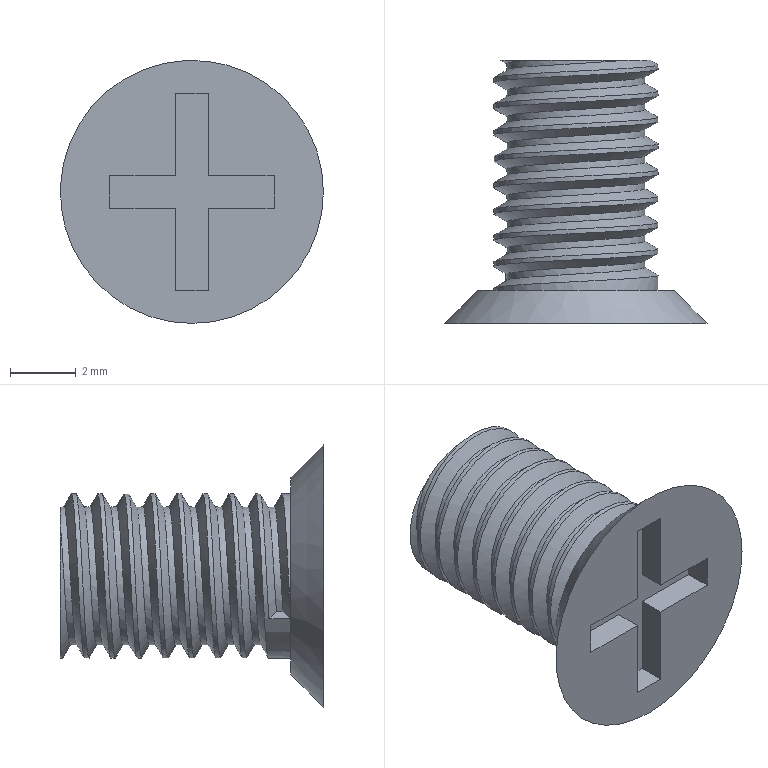Part | NX | features EXTRUDE 3, SKETCH 3, CHAMFER 1, DATUM_CSYS 1, THREADS 1, UNITE 1 | 1 solid | 23 faces | box 8 x 8 x 8 mm | volume 147.132 mm3 | plane 17 | spline 3 | cylinder 2 | cone 1 | commonest cylinder face diameters 4.2 x1 5 x1